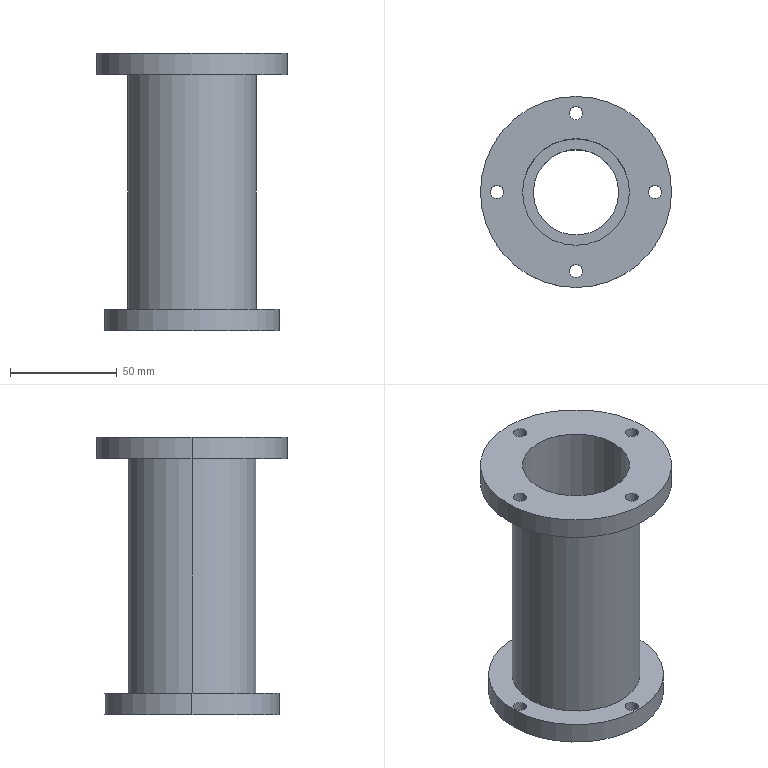Part | STEP file | Double-tube connecting pipe SGN-2-07 | 1 solid | 31 faces | box 89.5 x 89.5 x 130 mm | volume 204335 mm3 | cylinder 26 | plane 5 | commonest cylinder face diameters 6.3 x16 40 x2 50 x2 60 x2 82 x2 89.5 x2